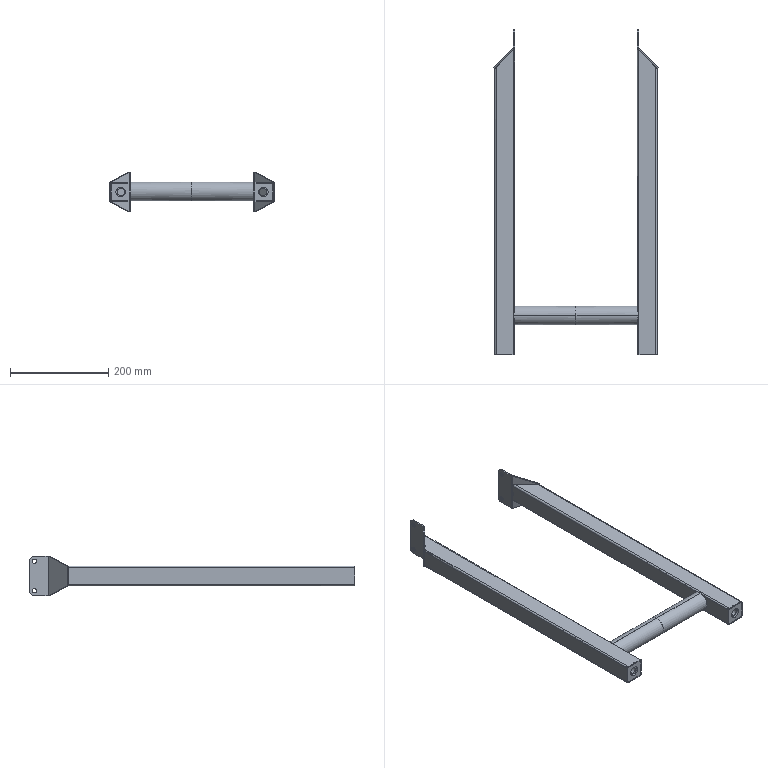Part | STEP file | MM-P46715-07_1 | 12 solids | 152 faces | box 334.243 x 661.5 x 80 mm | volume 460101 mm3 | plane 84 | cylinder 60 | spline 8 | commonest cylinder face diameters 2 x18 6 x12 9 x8 20 x8 14.5 x4 35 x4